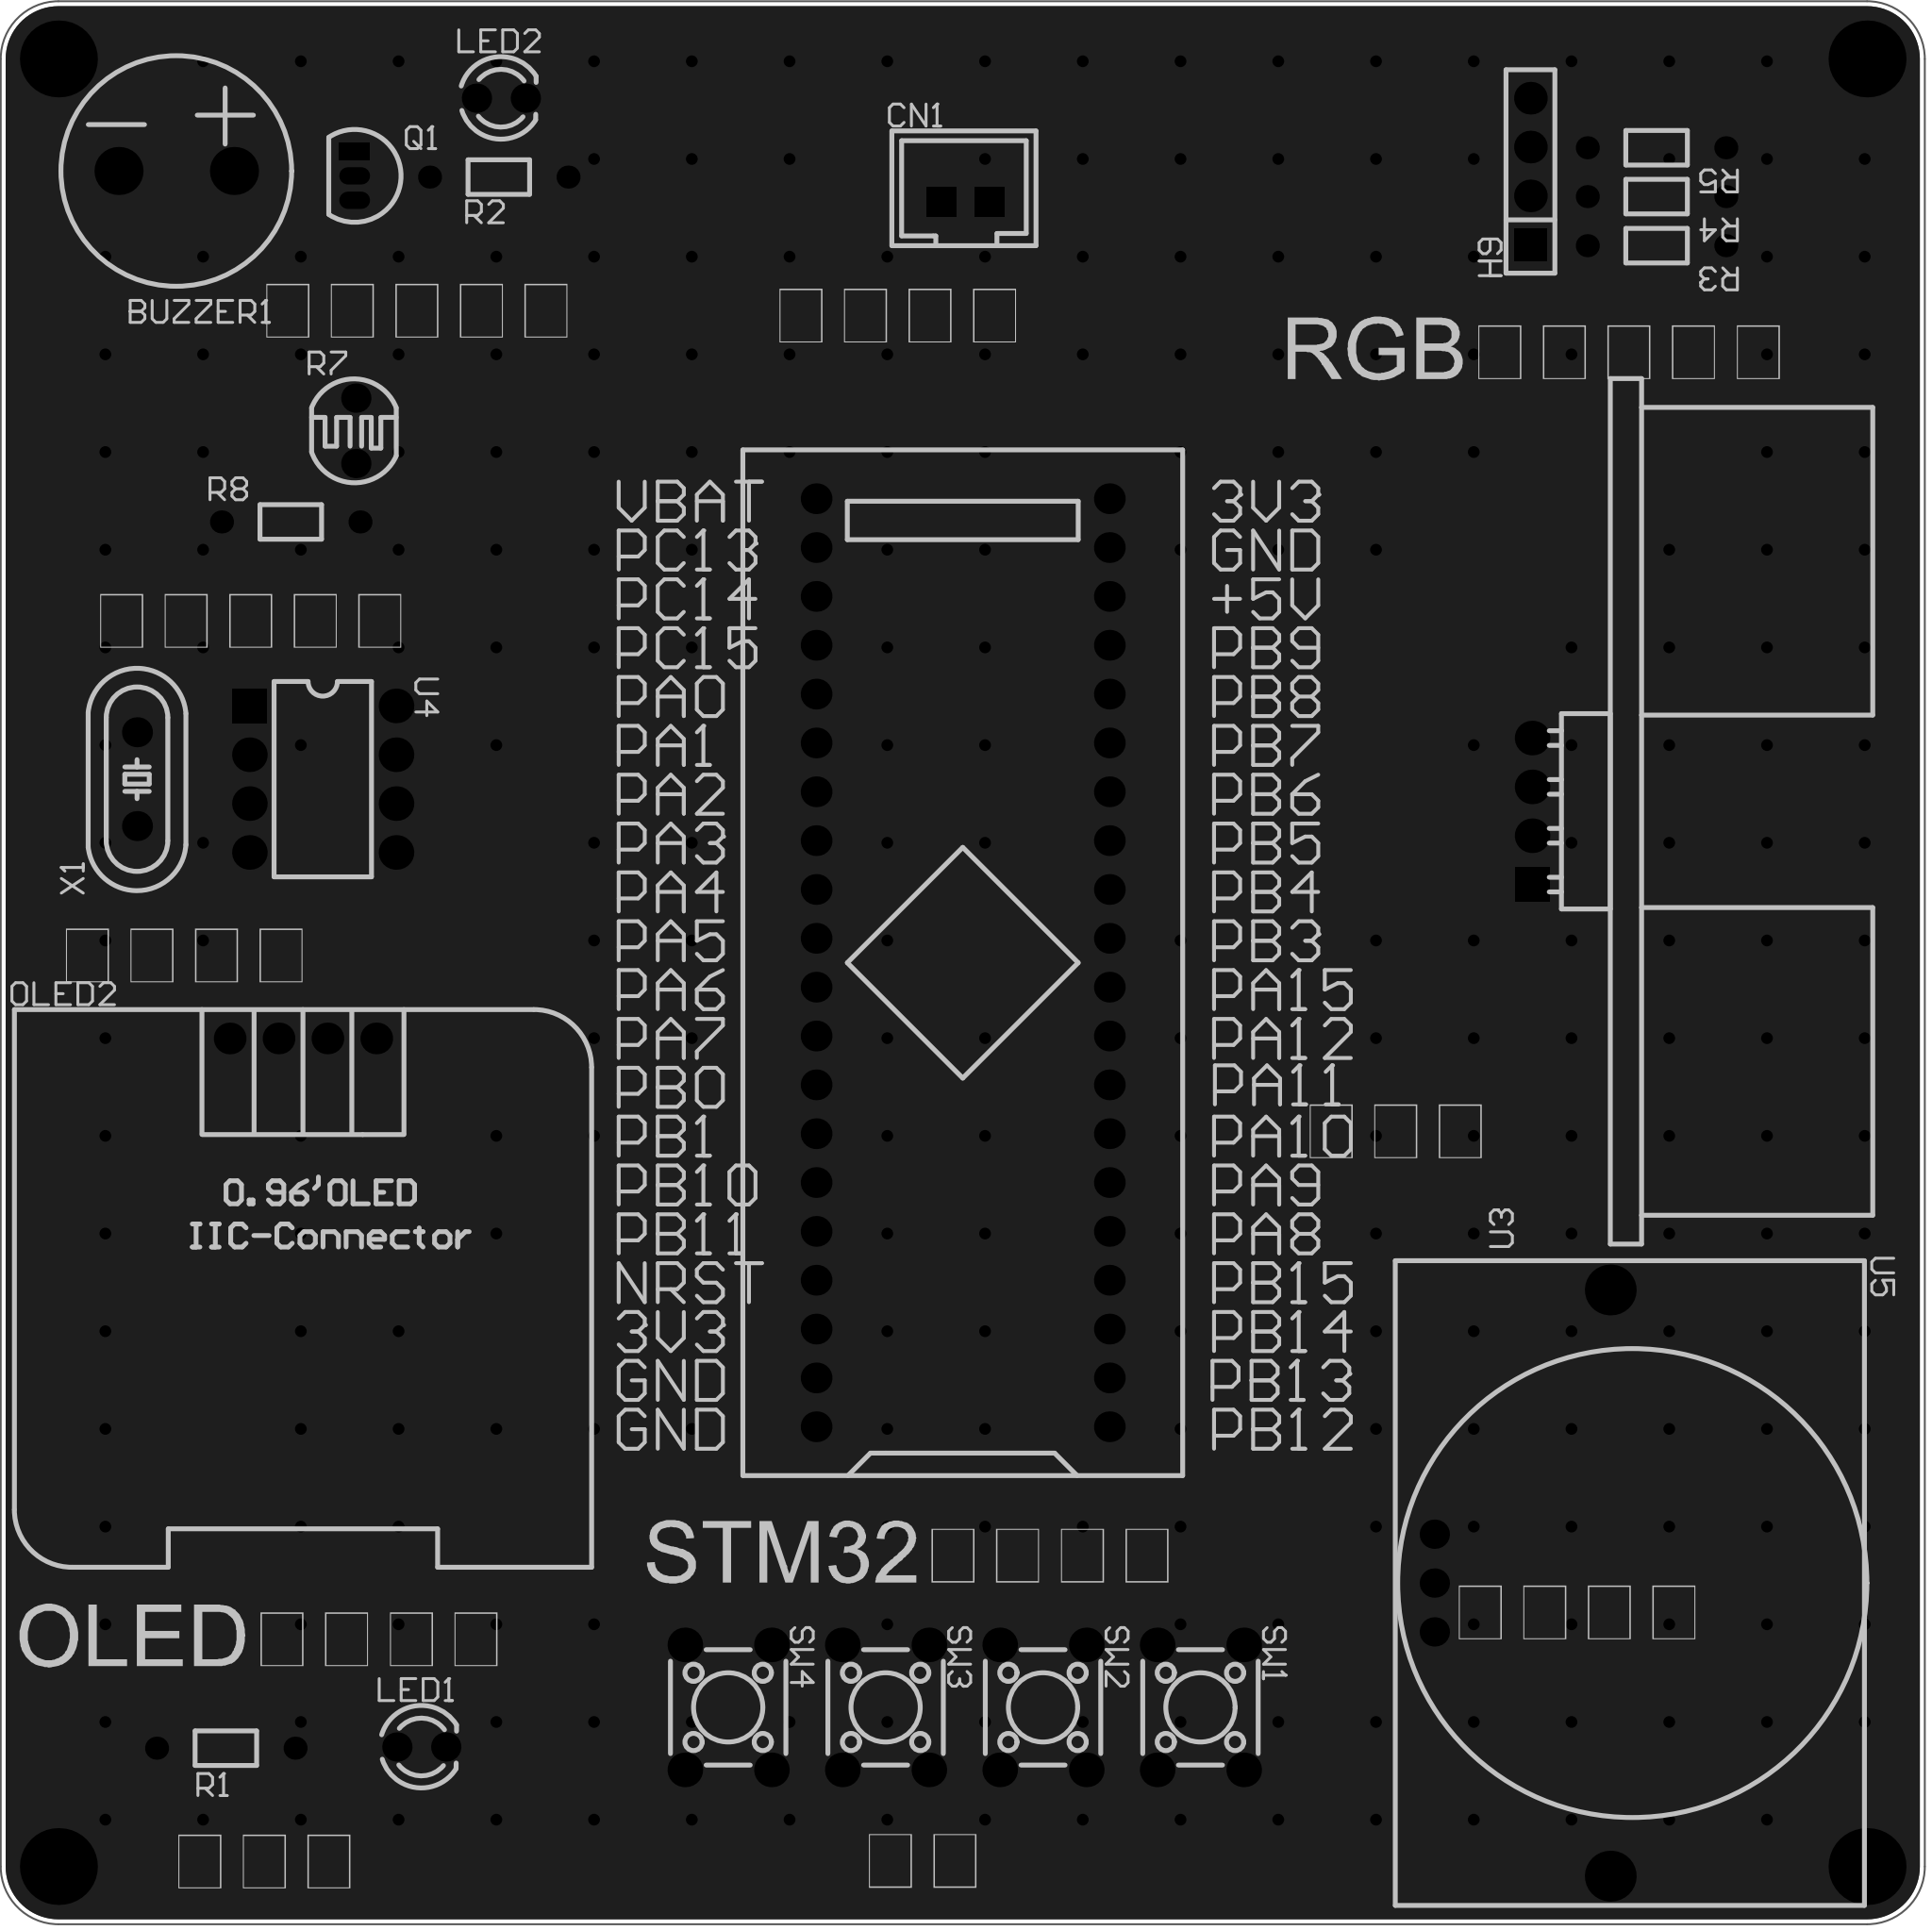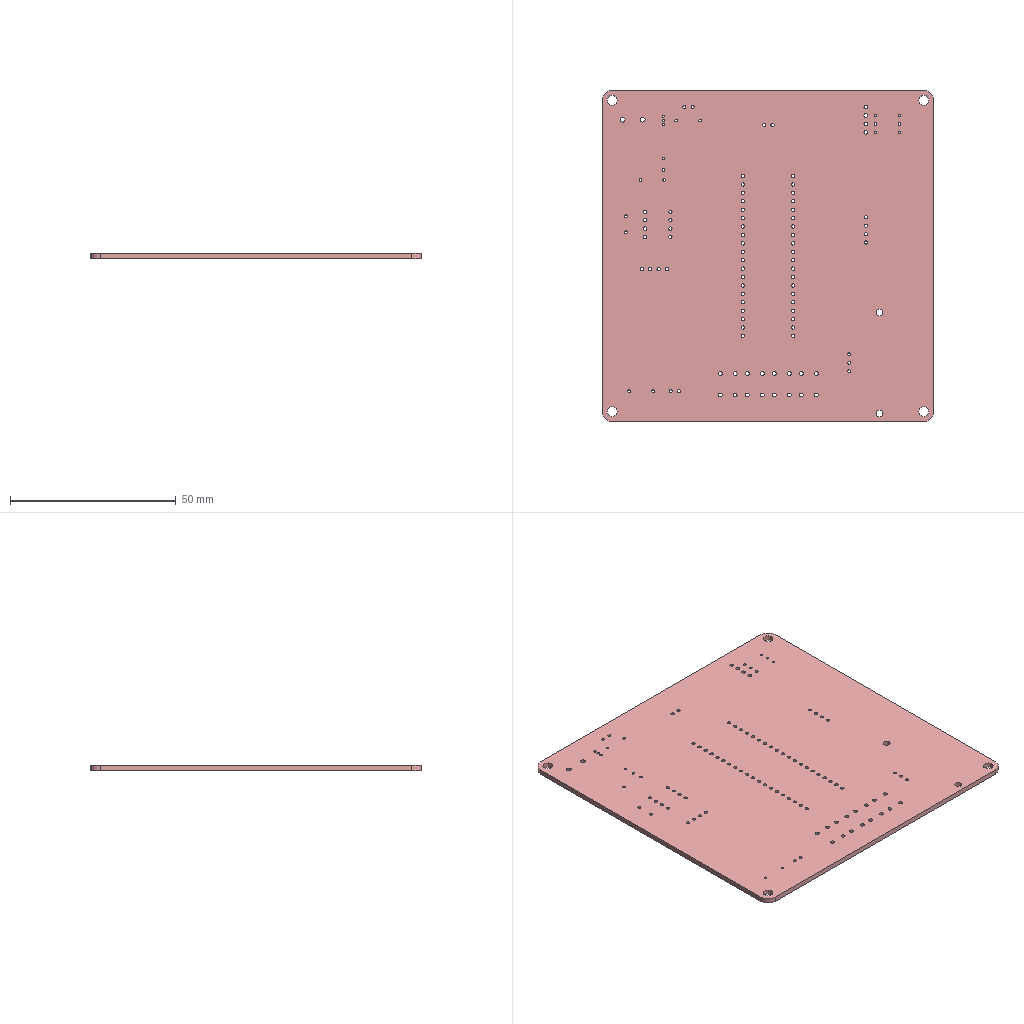Circuit board layout | Altium Designer | box 100 x 100 x 1.6 mm
Layer stack:
# Altium Designer layer stack of  (unit mm; dielectric type: 0 none, 1 core, 2 prepreg, 3 surface material)
index,name,kind,layer,copper_thickness_mm,dielectric_type,dielectric_thickness_mm,dielectric_material,dielectric_constant
0,Top Paste Mask Layer,other,,,,,,
1,Top Silkscreen Layer,other,,,,,,
2,Top Solder Mask Layer,dielectric,,,3,0.01,,3.3
3,Top Layer,copper,Top Layer,0.035,,,,
4,Dielectric1,dielectric,,,3,1.51,FR4,4.5
5,Bottom Layer,copper,Bottom Layer,0.035,,,,
6,Bottom Solder Mask Layer,dielectric,,,3,0.01,,3.3
7,Bottom Silkscreen Layer,other,,,,,,
8,Bottom Paste Mask Layer,other,,,,,,
# drill layer pairs: low layer,high layer
drill_pair,Top Layer,Bottom Layer
Part placement:
Designator,Comment,Layer,Footprint,Center-X(mm),Center-Y(mm),Rotation
U1,STM32F103C8T6-Card,TopLayer,CONN-TH_L53.3-W22.9_STM32F103C8T6-CARD,141.351,130.937,90
BUZZER1,buzzer,TopLayer,BUZ-TH_BD12.0-P6.00-D0.9-RD,100.475,172.111,0
H9,,TopLayer,HDR-TH_4P-P2.54-V-F,170.855,172.085,90
LED1,,TopLayer,LED_TH-3mm,113.212,90.155,0
LED2,,TopLayer,LED_TH-3mm,117.348,175.895,0
OLED2,,TopLayer,0.96OLED_4P,107.061,127,0
Q1,,TopLayer,S8050_TO_92,109.746,171.857,270
R1,10kΩ,TopLayer,Res_1/8W,103.052,90.092,180
R2,1kΩ,TopLayer,Res_1/8W,117.239,171.794,180
R3,100Ω,TopLayer,Res_1/8W,177.411,168.225,180
R4,100Ω,TopLayer,Res_1/8W,177.411,170.778,180
R5,100Ω,TopLayer,Res_1/8W,177.411,173.318,180
R7,GL5549(80-100),TopLayer,RES-TH_L5.1-W4.3-P3.40-D0.5,109.808,158.597,0
R8,10kΩ,TopLayer,Res_1/8W,106.426,153.86,0
SW1,,TopLayer,SW-TH_4P-L6.0-W6.0-P4.50-LS6.5,153.704,92.214,270
SW2,,TopLayer,SW-TH_4P-L6.0-W6.0-P4.50-LS6.5,145.523,92.214,270
SW3,,TopLayer,SW-TH_4P-L6.0-W6.0-P4.50-LS6.5,137.341,92.214,270
SW4,,TopLayer,SW-TH_4P-L6.0-W6.0-P4.50-LS6.5,129.159,92.214,270
U3,HC-SR04,TopLayer,TH_HC-SR04V,170.942,138.811,90
U4,DS1302N,TopLayer,DIP-8_L9.7-W6.4-P2.54-LS7.6-BL,108.088,140.483,270
U5,,TopLayer,HC-SR501,170.434,98.679,270
X1,32.768KHZ,TopLayer,HC-49S_L11.5-W5.0-P4.88,98.436,140.483,90
CN1,XH2.54-2PIN-直针,TopLayer,CONN-TH_XH2.54-2P,141.476,170.512,0
Pad and via stacks:
# Altium Designer via and pad stacks of  (unit mm). Each distinct definition once, with the count of objects using it.
# via: kind,start_layer,end_layer,hole_mm,diameter_mm,mode(0 simple;1 top-mid-bottom;2 full stack),diameter_per_layer,count,example_net
# pad: kind,layer,hole_mm,hole_type(0 round;1 square;2 slot),plating,top_size,top_shape(1 round;2 rect;3 octagon;9 rounded rect),mid_size,bottom_size,mode,footprint,size_per_layer,count,example
pad,Multi-Layer,3,0,plated,4x4,1,4x4,4x4,0,,,4,1
pad,Multi-Layer,1,0,plated,1.6x1.6,1,1.6x1.6,1.6x1.6,0,CONN-TH_L53.3-W22.9_STM32F103C8T6-CARD,,40,U1.1
pad,Multi-Layer,1.5,0,plated,2.5x2.5,1,2.5x2.5,2.5x2.5,0,BUZ-TH_BD12.0-P6.00-D0.9-RD,,2,BUZZER1.1
pad,Multi-Layer,1.1,0,plated,1.7x1.7,2,1.7x1.7,1.7x1.7,0,HDR-TH_4P-P2.54-V-F,,1,H9.1
pad,Multi-Layer,1.1,0,plated,1.7x1.7,1,1.7x1.7,1.7x1.7,0,HDR-TH_4P-P2.54-V-F,,3,H9.2
pad,Multi-Layer,0.9144,0,plated,1.524x1.524,1,1.524x1.524,1.524x1.524,0,LED_TH-3mm,,4,LED1.1
pad,Multi-Layer,1,0,plated,1.65x1.65,1,1.65x1.65,1.65x1.65,0,0.96OLED_4P,,4,OLED2.4
pad,Multi-Layer,0.701,0,plated,0.8992x1.6,2,0.8992x1.6,0.8992x1.6,0,S8050_TO_92,,1,Q1.1
pad,Multi-Layer,0.701,0,plated,0.8992x1.6,1,0.8992x1.6,0.8992x1.6,0,S8050_TO_92,,2,Q1.2
pad,Multi-Layer,0.8001,0,plated,1.199x1.199,1,1.199x1.199,1.199x1.199,0,Res_1/8W,,12,R1.1
pad,Multi-Layer,0.762,0,plated,1.524x1.524,1,1.524x1.524,1.524x1.524,0,RES-TH_L5.1-W4.3-P3.40-D0.5,,2,R7.2
pad,Multi-Layer,1.2,0,plated,1.8x1.8,1,1.8x1.8,1.8x1.8,0,SW-TH_4P-L6.0-W6.0-P4.50-LS6.5,,16,SW1.1
pad,Multi-Layer,1.001,0,plated,1.8x1.8,1,1.8x1.8,1.8x1.8,0,TH_HC-SR04V,,3,U3.4
pad,Multi-Layer,1.001,0,plated,1.8x1.8,2,1.8x1.8,1.8x1.8,0,TH_HC-SR04V,,1,U3.1
pad,Multi-Layer,1,0,plated,1.8x1.8,2,1.8x1.8,1.8x1.8,0,DIP-8_L9.7-W6.4-P2.54-LS7.6-BL,,1,U4.1
pad,Multi-Layer,1,0,plated,1.8x1.8,1,1.8x1.8,1.8x1.8,0,DIP-8_L9.7-W6.4-P2.54-LS7.6-BL,,7,U4.2
pad,Multi-Layer,2.032,0,plated,2.642x2.642,1,2.642x2.642,2.642x2.642,0,HC-SR501,,2,U5.
pad,Multi-Layer,0.914,0,plated,1.524x1.524,1,1.524x1.524,1.524x1.524,0,HC-SR501,,3,U5.1
pad,Multi-Layer,0.9,0,plated,1.56x1.56,1,1.56x1.56,1.56x1.56,0,HC-49S_L11.5-W5.0-P4.88,,2,X1.1
pad,Multi-Layer,1,2,plated,1.524x1.524,2,1.524x1.524,1.524x1.524,0,CONN-TH_XH2.54-2P,,2,CN1.1
via,Top Layer,Bottom Layer,0.3048,0.61,0,,263,GND
Copper pours:
name,layer,net,type(0 solid;1 hatched;2 none)
Bottom Layer-GND,Bottom Layer,GND,0
Top Layer-GND,Top Layer,GND,0
Design rules, without the lines most boards share:
# Altium Designer design rules of  (exported by Altium Designer, unit mm)
# columns: name | kind | enabled | priority | scope1 | scope2 | descriptor | typed fields (field=value)
Copper_copperRegion_copperThickness1oz | 0 | disabled | 4 | All | All | Clearance Constraint (Gap=5.984mil) (Disabled)(All),(All) | gap=0.152
Copper_copperRegion_copperThickness1oz_1 | 63 | disabled | 4 | All | All | Board Clearance Constraint (Gap=0mil) (Disabled)(All) |
Copper_copperRegion_Copper_copperRegion | 0 | disabled | 5 | All | All | Clearance Constraint (Gap=5.984mil) (Disabled)(All),(All) | gap=0.152
Copper_copperRegion_Copper_copperRegion_1 | 63 | disabled | 5 | All | All | Board Clearance Constraint (Gap=0mil) (Disabled)(All) |
copperThickness1oz | 0 | enabled | 6 | All | All | Clearance Constraint (Gap=5.984mil) (All),(All) | gap=0.152
copperThickness1oz_1 | 63 | enabled | 6 | All | All | Board Clearance Constraint (Gap=0mil) (All) |
copperRegion_copperThickness1oz | 20 | disabled | 1 | All | All | Polygon Connect Rule(Relief Connect )(Conductor Width=10mil) (Relief Angle=90 Angle) (Entries=4) (Air Gap Width=10mil) (Disabled)(All),(All) | connect_style(0=relief,1=direct,2=none)=0 relief_conductor_width=0.254 relief_entries=4
copperRegion_Copper_copperRegion | 20 | disabled | 2 | All | All | Polygon Connect Rule(Relief Connect )(Conductor Width=10mil) (Relief Angle=90 Angle) (Entries=4) (Air Gap Width=10mil) (Disabled)(All),(All) | connect_style(0=relief,1=direct,2=none)=0 relief_conductor_width=0.254 relief_entries=4
copperRegion | 20 | enabled | 3 | All | All | Polygon Connect Rule(Relief Connect )(Conductor Width=10mil) (Relief Angle=90 Angle) (Entries=4) (Air Gap Width=10mil) (All),(All) | connect_style(0=relief,1=direct,2=none)=0 relief_conductor_width=0.254 relief_entries=4